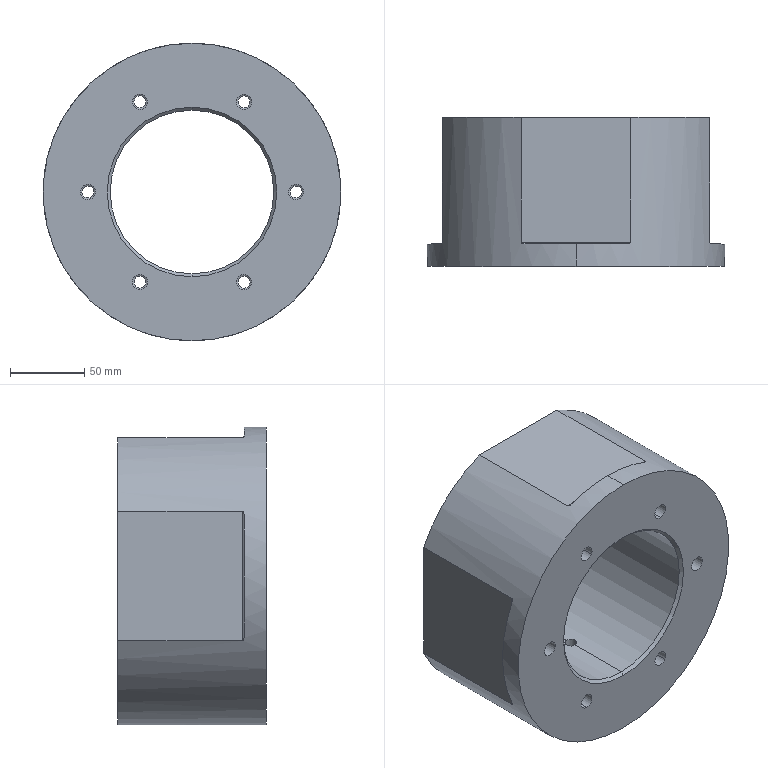Part | SolidWorks | features HoleWzd 5, ICE 3, 3DProfileFeature 1, Chamfer 1, CirPattern 1, Extrusion 1, Fillet 1 | 1 solid | 93 faces | box 200 x 100 x 200 mm | volume 2011529 mm3 | cylinder 53 | cone 32 | plane 8 | commonest cylinder face diameters 10.2 x24 8 x20 2 x3 11.8 x2 110 x2 200 x2